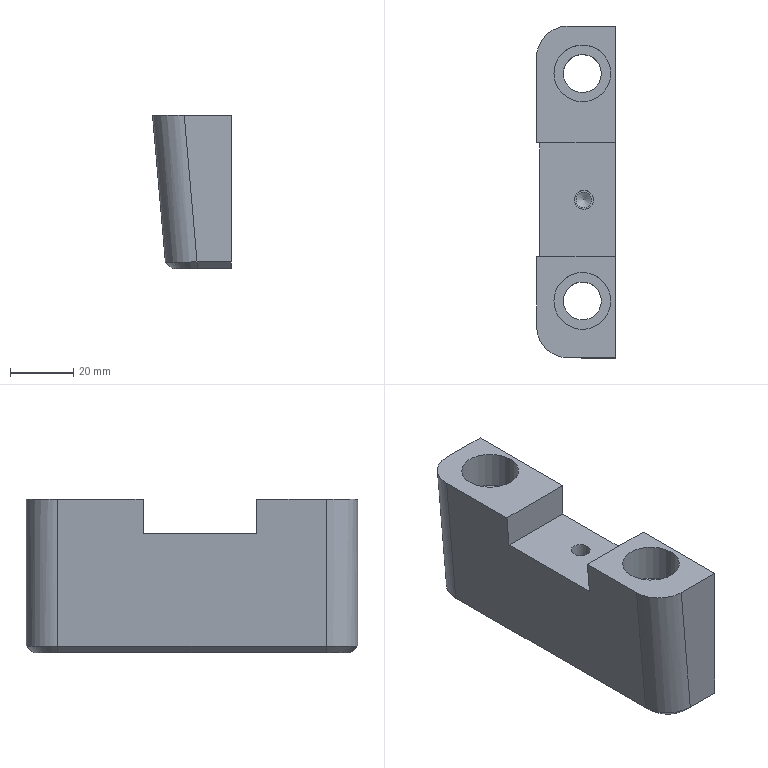Part | STEP file | solid 76 | 1 solid | 27 faces | box 25 x 105 x 48.598 mm | volume 89861 mm3 | plane 16 | cylinder 8 | spline 2 | cone 1 | commonest cylinder face diameters 12 x2 18 x2 20 x2 5 x1 6 x1